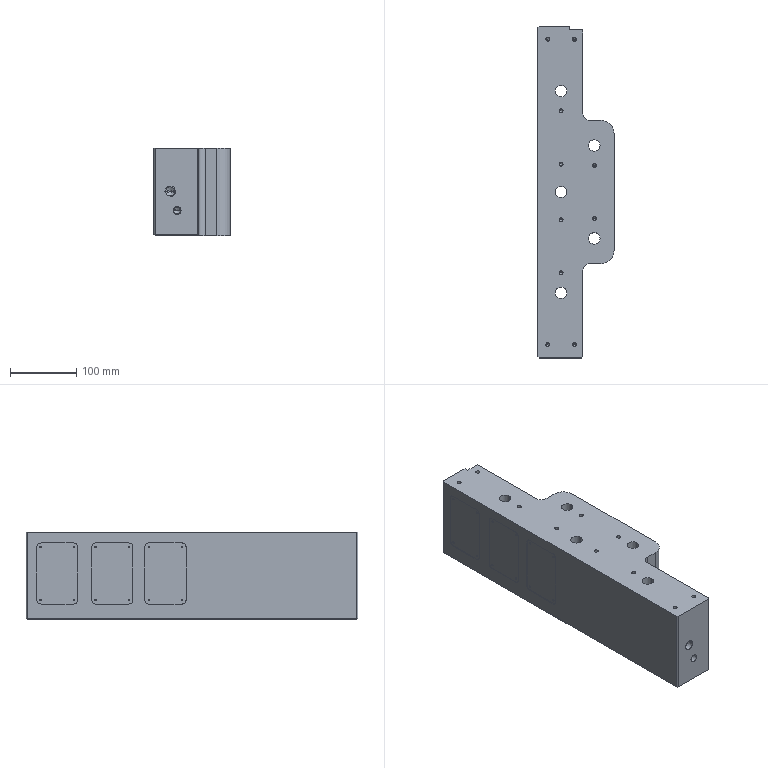Part | Creo | 2 solids | 377 faces | box 115 x 500 x 132 mm | volume 5598084 mm3 | cylinder 114 | plane 99 | cone 84 | other 80 | commonest cylinder face diameters 2.5 x24 4.97 x24 6 x24 12 x10 17.4 x10 10.5 x4